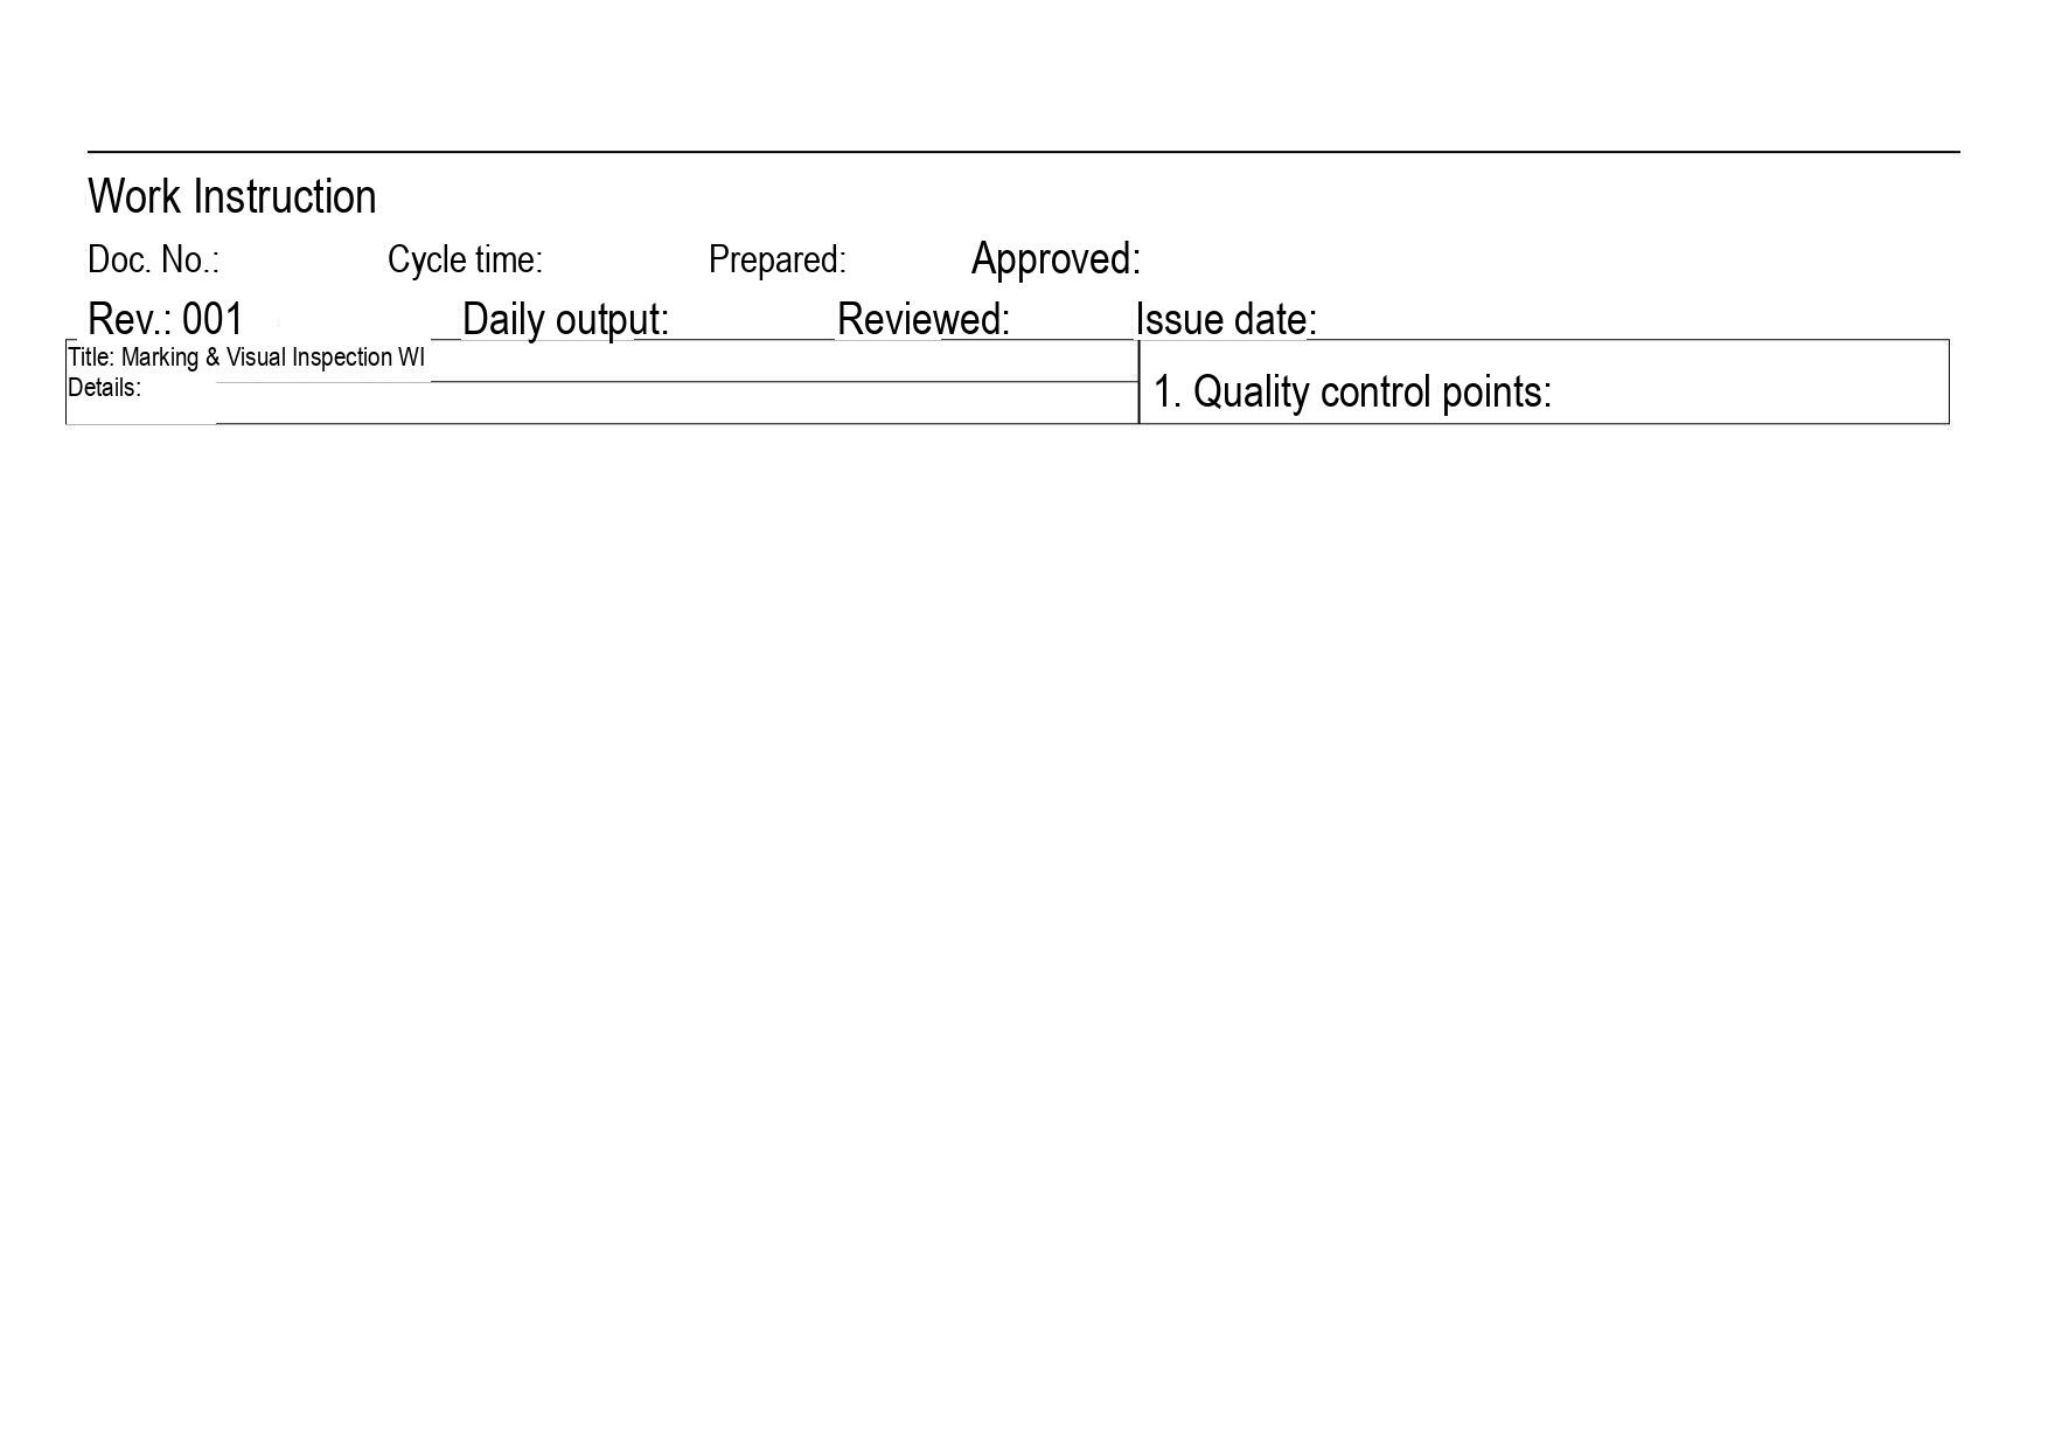Work Instruction

Doc. No.: Cycle time: Prepared: Approved:

Rev.: 001 Daily output: Reviewed: Issue date:

| Title: Marking & Visual Inspection WI<br>Details: | 1. Quality control points: |
|---|---|
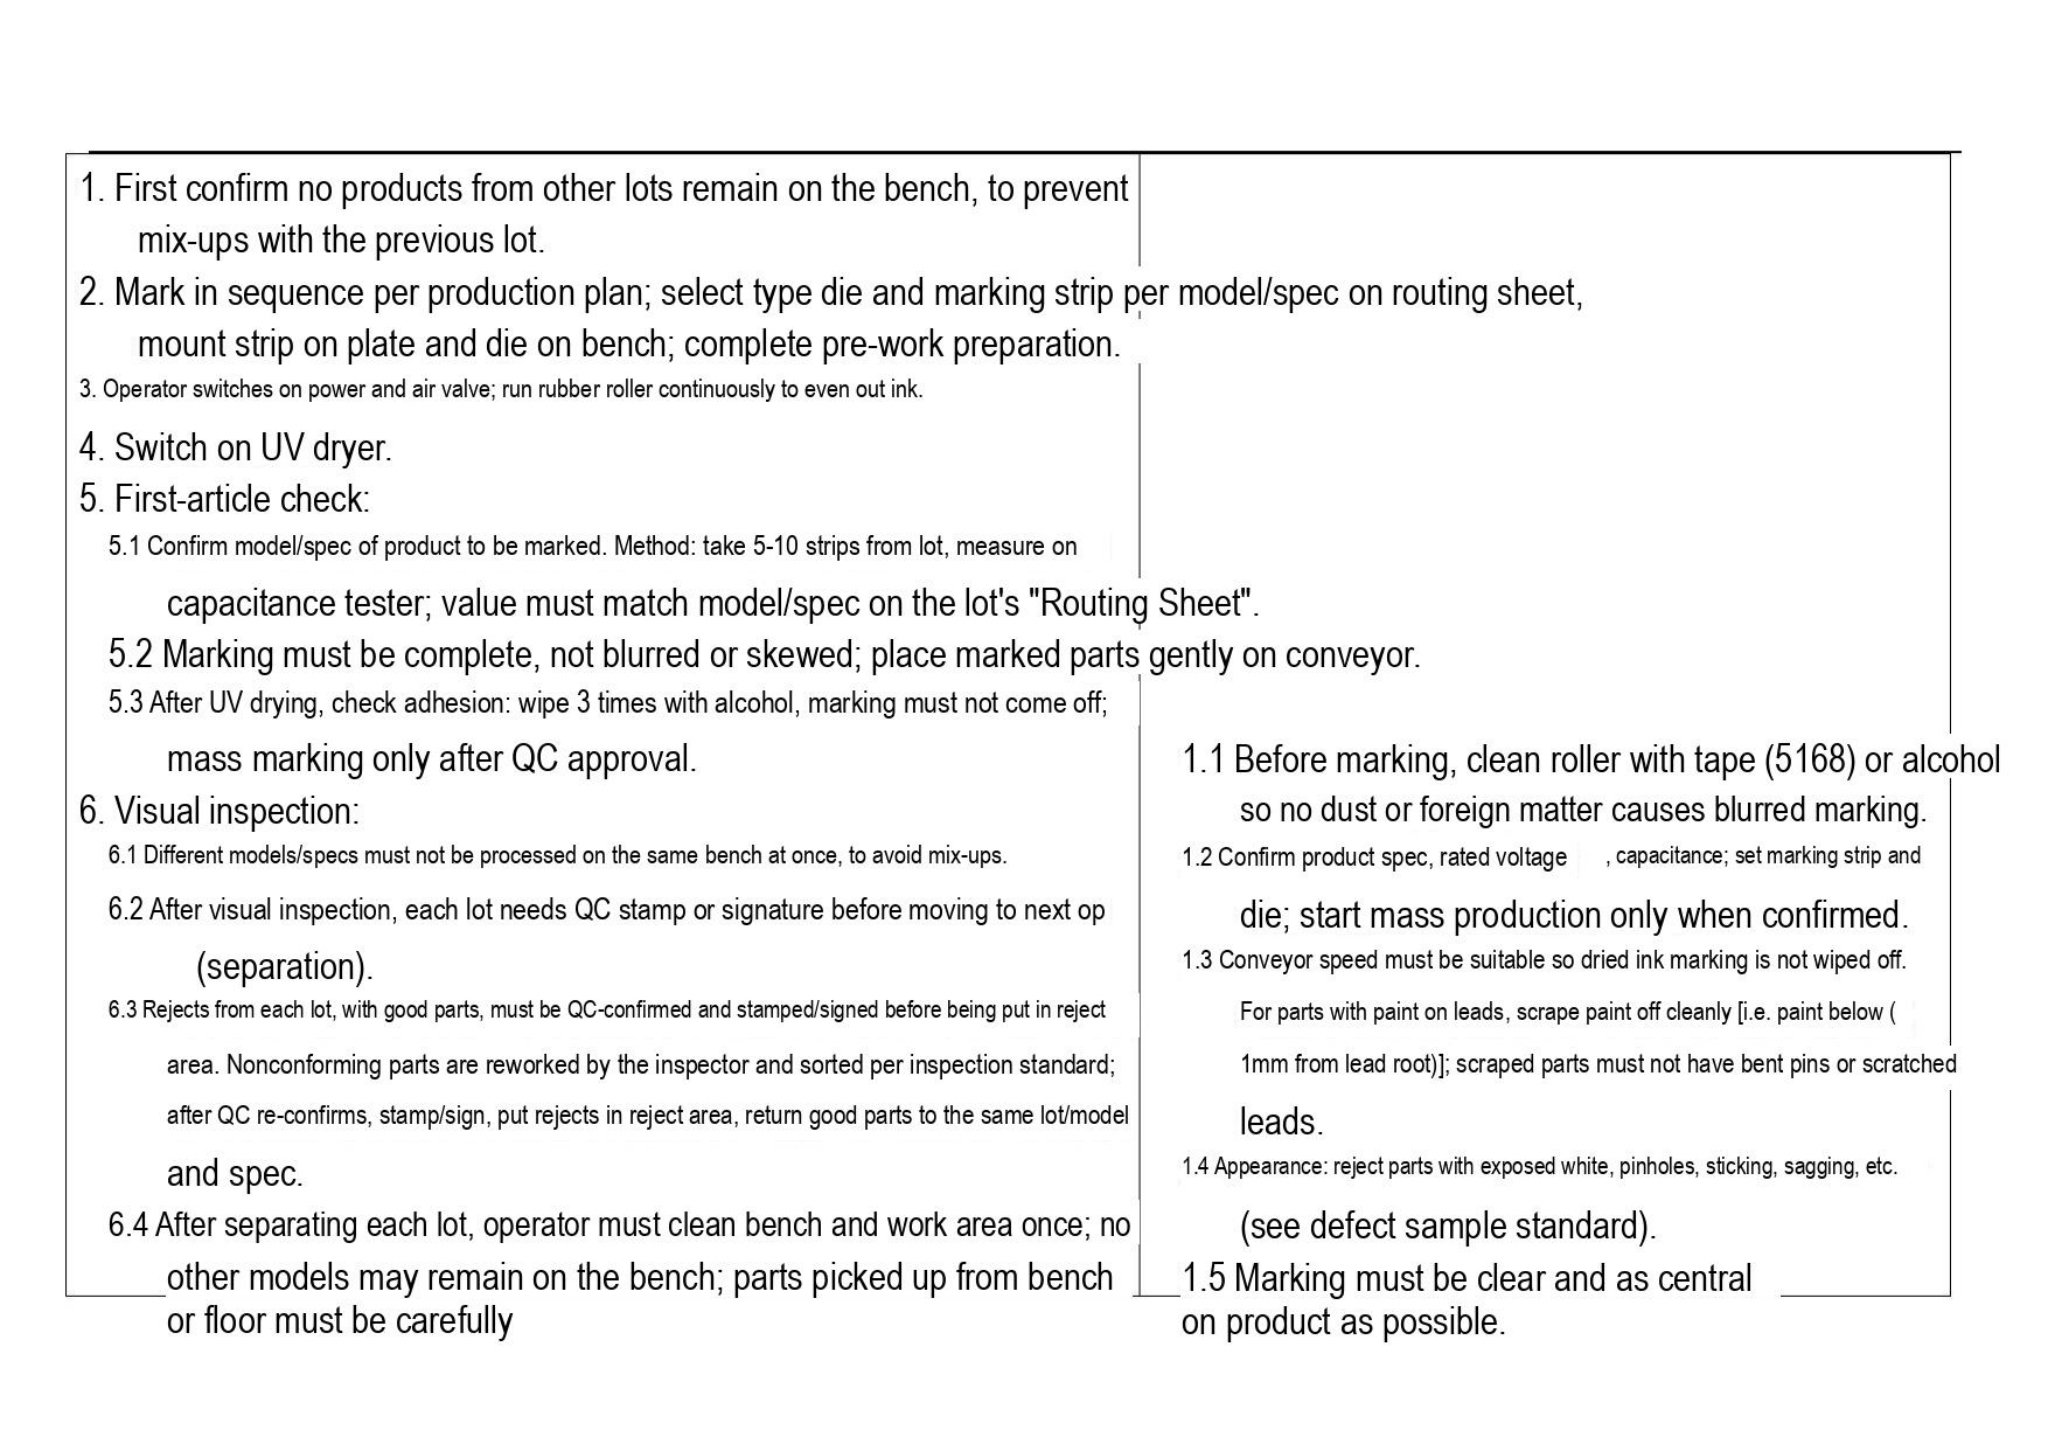1. First confirm no products from other lots remain on the bench, to prevent mix-ups with the previous lot.
2. Mark in sequence per production plan; select type die and marking strip per model/spec on routing sheet, mount strip on plate and die on bench; complete pre-work preparation.
3. Operator switches on power and air valve; run rubber roller continuously to even out ink.
4. Switch on UV dryer.
5. First-article check:
5.1 Confirm model/spec of product to be marked. Method: take 5-10 strips from lot, measure on capacitance tester; value must match model/spec on the lot's "Routing Sheet".
5.2 Marking must be complete, not blurred or skewed; place marked parts gently on conveyor.
5.3 After UV drying, check adhesion: wipe 3 times with alcohol, marking must not come off; mass marking only after QC approval.
6. Visual inspection:
6.1 Different models/specs must not be processed on the same bench at once, to avoid mix-ups.
6.2 After visual inspection, each lot needs QC stamp or signature before moving to next op (separation).
6.3 Rejects from each lot, with good parts, must be QC-confirmed and stamped/signed before being put in reject area. Nonconforming parts are reworked by the inspector and sorted per inspection standard; after QC re-confirms, stamp/sign, put rejects in reject area, return good parts to the same lot/model and spec.
6.4 After separating each lot, operator must clean bench and work area once; no other models may remain on the bench; parts picked up from bench or floor must be carefully

1.1 Before marking, clean roller with tape (5168) or alcohol so no dust or foreign matter causes blurred marking.
1.2 Confirm product spec, rated voltage , capacitance; set marking strip and die; start mass production only when confirmed.
1.3 Conveyor speed must be suitable so dried ink marking is not wiped off. For parts with paint on leads, scrape paint off cleanly [i.e. paint below ( 1mm from lead root)]; scraped parts must not have bent pins or scratched leads.
1.4 Appearance: reject parts with exposed white, pinholes, sticking, sagging, etc. (see defect sample standard).
1.5 Marking must be clear and as central on product as possible.
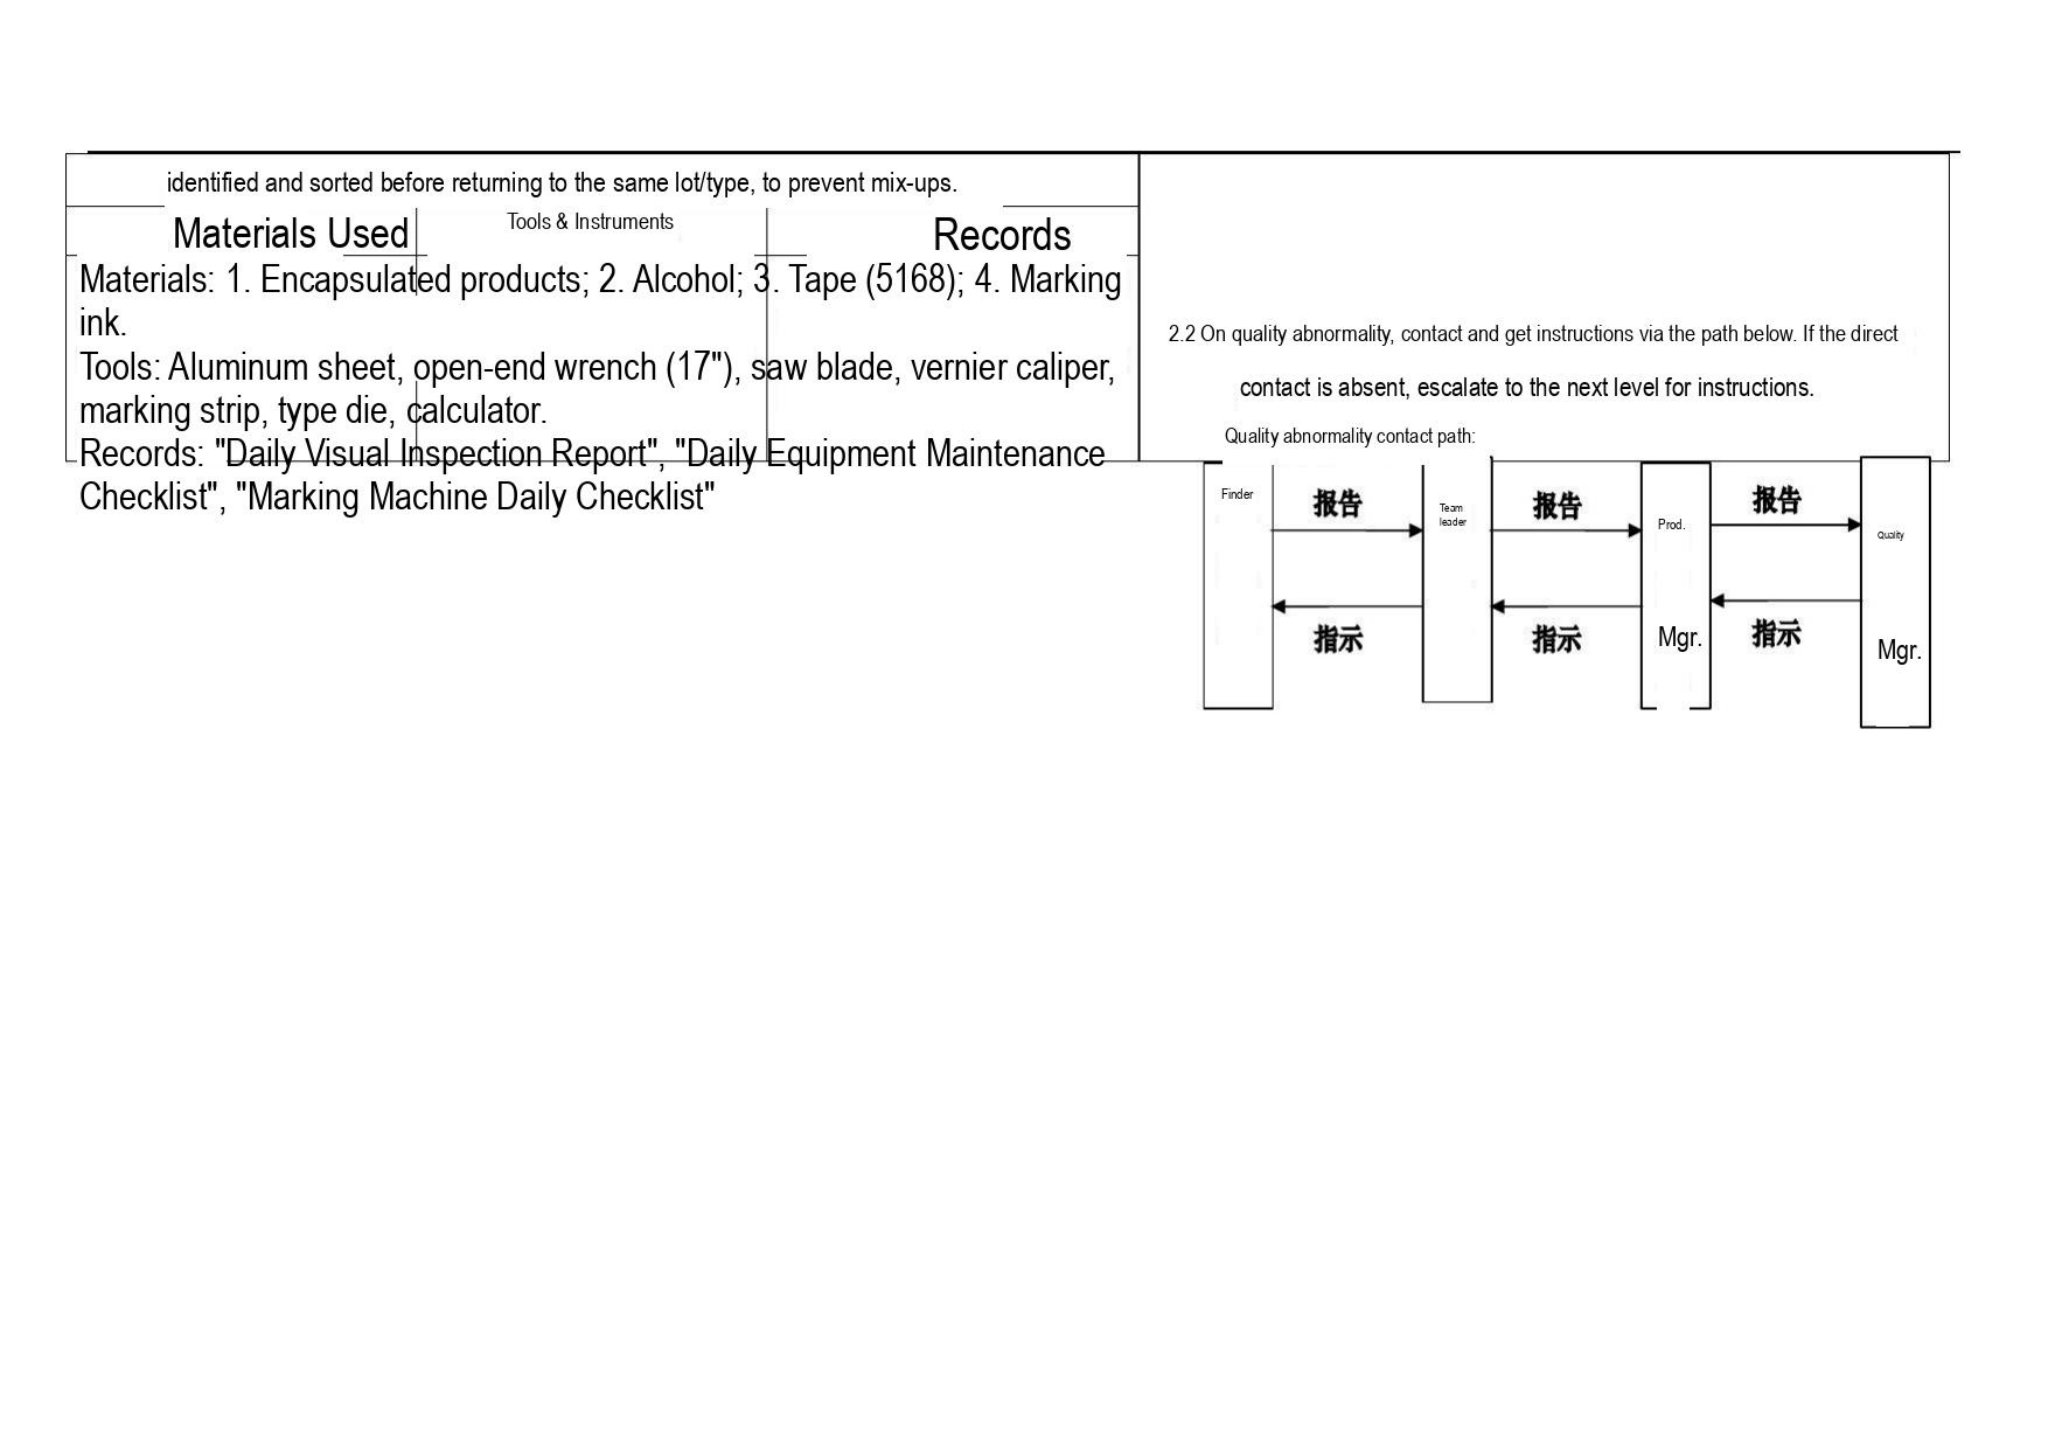identified and sorted before returning to the same lot/type, to prevent mix-ups.

| Materials Used | Tools & Instruments | Records |
|---|---|---|

Materials: 1. Encapsulated products; 2. Alcohol; 3. Tape (5168); 4. Marking ink.
Tools: Aluminum sheet, open-end wrench (17"), saw blade, vernier caliper, marking strip, type die, calculator.
Records: "Daily Visual Inspection Report", "Daily Equipment Maintenance Checklist", "Marking Machine Daily Checklist"

2.2 On quality abnormality, contact and get instructions via the path below. If the direct contact is absent, escalate to the next level for instructions.

Quality abnormality contact path:

Finder
报告
指示
Team leader
报告
指示
Prod. Mgr.
报告
指示
Quality Mgr.